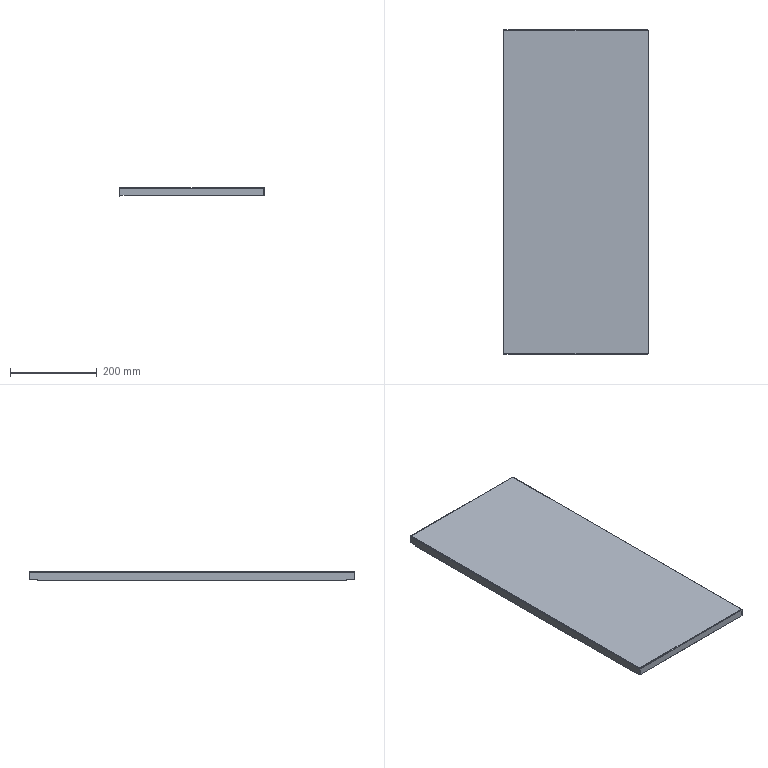Part | SolidWorks | features BaseBody 1 | 1 solid | 44 faces | box 336 x 750 x 20 mm | volume 346440 mm3 | plane 32 | cylinder 8 | spline 4 | commonest cylinder face diameters 1 x4 3.4 x4
STEP:
#1=CARTESIAN_POINT('',(-168.,-375.,-18.));
#2=VERTEX_POINT('',#1);
#3=CARTESIAN_POINT('',(-168.,-357.,-18.));
#4=VERTEX_POINT('',#3);
#5=CARTESIAN_POINT('',(-168.,-375.,-18.));
#6=DIRECTION('',(0.,1.,0.));
#7=VECTOR('',#6,1000.);
#8=LINE('',#5,#7);
#9=EDGE_CURVE('',#2,#4,#8,.T.);
#10=ORIENTED_EDGE('',*,*,#9,.T.);
#11=CARTESIAN_POINT('',(-166.8,-357.,-18.));
#12=VERTEX_POINT('',#11);
#13=CARTESIAN_POINT('',(-166.8,-357.,-18.));
#14=DIRECTION('',(-1.,0.,0.));
#15=VECTOR('',#14,1000.);
#16=LINE('',#13,#15);
#17=EDGE_CURVE('',#12,#4,#16,.T.);
#18=ORIENTED_EDGE('',*,*,#17,.F.);
#19=CARTESIAN_POINT('',(-166.8,-375.,-18.));
#20=VERTEX_POINT('',#19);
#21=CARTESIAN_POINT('',(-166.8,-375.,-18.));
#22=DIRECTION('',(0.,1.,0.));
#23=VECTOR('',#22,1000.);
#24=LINE('',#21,#23);
#25=EDGE_CURVE('',#20,#12,#24,.T.);
#26=ORIENTED_EDGE('',*,*,#25,.F.);
#27=CARTESIAN_POINT('',(-166.8,-375.,-18.));
#28=DIRECTION('',(-1.,0.,0.));
#29=VECTOR('',#28,1000.);
#30=LINE('',#27,#29);
#31=EDGE_CURVE('',#20,#2,#30,.T.);
#32=ORIENTED_EDGE('',*,*,#31,.T.);
#33=EDGE_LOOP('',(#10,#18,#26,#32));
#34=FACE_OUTER_BOUND('',#33,.T.);
#35=CARTESIAN_POINT('',(-166.8,-375.,-18.));
#36=DIRECTION('',(0.,0.,1.));
#37=DIRECTION('',(1.,0.,0.));
#38=AXIS2_PLACEMENT_3D('',#35,#36,#37);
#39=PLANE('',#38);
#40=ADVANCED_FACE('',(#34),#39,.F.);
#41=CARTESIAN_POINT('',(-168.,-357.,-20.));
#42=VERTEX_POINT('',#41);
#43=CARTESIAN_POINT('',(-168.,-357.,-20.));
#44=DIRECTION('',(0.,0.,-1.));
#45=VECTOR('',#44,1000.);
#46=LINE('',#43,#45);
#47=EDGE_CURVE('',#4,#42,#46,.T.);
#48=ORIENTED_EDGE('',*,*,#47,.T.);
#49=CARTESIAN_POINT('',(-166.8,-357.,-20.));
#50=VERTEX_POINT('',#49);
#51=CARTESIAN_POINT('',(-166.8,-357.,-20.));
#52=DIRECTION('',(-1.,0.,0.));
#53=VECTOR('',#52,1000.);
#54=LINE('',#51,#53);
#55=EDGE_CURVE('',#50,#42,#54,.T.);
#56=ORIENTED_EDGE('',*,*,#55,.F.);
#57=CARTESIAN_POINT('',(-166.8,-357.,-20.));
#58=DIRECTION('',(0.,0.,-1.));
#59=VECTOR('',#58,1000.);
#60=LINE('',#57,#59);
#61=EDGE_CURVE('',#12,#50,#60,.T.);
#62=ORIENTED_EDGE('',*,*,#61,.F.);
#63=ORIENTED_EDGE('',*,*,#17,.T.);
#64=EDGE_LOOP('',(#48,#56,#62,#63));
#65=FACE_OUTER_BOUND('',#64,.T.);
#66=CARTESIAN_POINT('',(-166.8,-357.,-20.));
#67=DIRECTION('',(0.,1.,0.));
#68=DIRECTION('',(1.,0.,0.));
#69=AXIS2_PLACEMENT_3D('',#66,#67,#68);
#70=PLANE('',#69);
#71=ADVANCED_FACE('',(#65),#70,.F.);
#72=CARTESIAN_POINT('',(-168.,357.,-20.));
#73=VERTEX_POINT('',#72);
#74=CARTESIAN_POINT('',(-168.,357.,-18.));
#75=VERTEX_POINT('',#74);
#76=CARTESIAN_POINT('',(-168.,357.,-20.));
#77=DIRECTION('',(0.,0.,1.));
#78=VECTOR('',#77,1000.);
#79=LINE('',#76,#78);
#80=EDGE_CURVE('',#73,#75,#79,.T.);
#81=ORIENTED_EDGE('',*,*,#80,.T.);
#82=CARTESIAN_POINT('',(-166.8,357.,-18.));
#83=VERTEX_POINT('',#82);
#84=CARTESIAN_POINT('',(-166.8,357.,-18.));
#85=DIRECTION('',(-1.,0.,0.));
#86=VECTOR('',#85,1000.);
#87=LINE('',#84,#86);
#88=EDGE_CURVE('',#83,#75,#87,.T.);
#89=ORIENTED_EDGE('',*,*,#88,.F.);
#90=CARTESIAN_POINT('',(-166.8,357.,-20.));
#91=VERTEX_POINT('',#90);
#92=CARTESIAN_POINT('',(-166.8,357.,-20.));
#93=DIRECTION('',(0.,0.,1.));
#94=VECTOR('',#93,1000.);
#95=LINE('',#92,#94);
#96=EDGE_CURVE('',#91,#83,#95,.T.);
#97=ORIENTED_EDGE('',*,*,#96,.F.);
#98=CARTESIAN_POINT('',(-166.8,357.,-20.));
#99=DIRECTION('',(-1.,0.,0.));
#100=VECTOR('',#99,1000.);
#101=LINE('',#98,#100);
#102=EDGE_CURVE('',#91,#73,#101,.T.);
#103=ORIENTED_EDGE('',*,*,#102,.T.);
#104=EDGE_LOOP('',(#81,#89,#97,#103));
#105=FACE_OUTER_BOUND('',#104,.T.);
#106=CARTESIAN_POINT('',(-166.8,357.,-20.));
#107=DIRECTION('',(0.,-1.,0.));
#108=DIRECTION('',(0.,0.,-1.));
#109=AXIS2_PLACEMENT_3D('',#106,#107,#108);
#110=PLANE('',#109);
#111=ADVANCED_FACE('',(#105),#110,.F.);
#112=CARTESIAN_POINT('',(-168.,375.,-18.));
#113=VERTEX_POINT('',#112);
#114=CARTESIAN_POINT('',(-168.,375.,-18.));
#115=DIRECTION('',(0.,1.,0.));
#116=VECTOR('',#115,1000.);
#117=LINE('',#114,#116);
#118=EDGE_CURVE('',#75,#113,#117,.T.);
#119=ORIENTED_EDGE('',*,*,#118,.T.);
#120=CARTESIAN_POINT('',(-166.8,375.,-18.));
#121=VERTEX_POINT('',#120);
#122=CARTESIAN_POINT('',(-166.8,375.,-18.));
#123=DIRECTION('',(-1.,0.,0.));
#124=VECTOR('',#123,1000.);
#125=LINE('',#122,#124);
#126=EDGE_CURVE('',#121,#113,#125,.T.);
#127=ORIENTED_EDGE('',*,*,#126,.F.);
#128=CARTESIAN_POINT('',(-166.8,375.,-18.));
#129=DIRECTION('',(0.,1.,0.));
#130=VECTOR('',#129,1000.);
#131=LINE('',#128,#130);
#132=EDGE_CURVE('',#83,#121,#131,.T.);
#133=ORIENTED_EDGE('',*,*,#132,.F.);
#134=ORIENTED_EDGE('',*,*,#88,.T.);
#135=EDGE_LOOP('',(#119,#127,#133,#134));
#136=FACE_OUTER_BOUND('',#135,.T.);
#137=CARTESIAN_POINT('',(-166.8,375.,-18.));
#138=DIRECTION('',(0.,0.,1.));
#139=DIRECTION('',(1.,0.,0.));
#140=AXIS2_PLACEMENT_3D('',#137,#138,#139);
#141=PLANE('',#140);
#142=ADVANCED_FACE('',(#136),#141,.F.);
#143=CARTESIAN_POINT('',(166.093,375.,-18.));
#144=VERTEX_POINT('',#143);
#145=CARTESIAN_POINT('',(166.093,373.8,-18.));
#146=VERTEX_POINT('',#145);
#147=CARTESIAN_POINT('',(166.093,375.,-18.));
#148=DIRECTION('',(0.,-1.,0.));
#149=VECTOR('',#148,1000.);
#150=LINE('',#147,#149);
#151=EDGE_CURVE('',#144,#146,#150,.T.);
#152=ORIENTED_EDGE('',*,*,#151,.F.);
#153=CARTESIAN_POINT('',(166.093,375.,-1.7));
#154=VERTEX_POINT('',#153);
#155=CARTESIAN_POINT('',(166.093,375.,0.));
#156=DIRECTION('',(0.,0.,-1.));
#157=VECTOR('',#156,1000.);
#158=LINE('',#155,#157);
#159=EDGE_CURVE('',#154,#144,#158,.T.);
#160=ORIENTED_EDGE('',*,*,#159,.F.);
#161=CARTESIAN_POINT('',(166.093,373.8,-1.7));
#162=VERTEX_POINT('',#161);
#163=CARTESIAN_POINT('',(166.093,373.8,-1.7));
#164=DIRECTION('',(0.,-1.,0.));
#165=VECTOR('',#164,1000.);
#166=LINE('',#163,#165);
#167=EDGE_CURVE('',#154,#162,#166,.T.);
#168=ORIENTED_EDGE('',*,*,#167,.T.);
#169=CARTESIAN_POINT('',(166.093,373.8,-1.2));
#170=DIRECTION('',(0.,0.,-1.));
#171=VECTOR('',#170,1000.);
#172=LINE('',#169,#171);
#173=EDGE_CURVE('',#162,#146,#172,.T.);
#174=ORIENTED_EDGE('',*,*,#173,.T.);
#175=EDGE_LOOP('',(#152,#160,#168,#174));
#176=FACE_OUTER_BOUND('',#175,.T.);
#177=CARTESIAN_POINT('',(166.093,373.8,-1.2));
#178=DIRECTION('',(-1.,0.,0.));
#179=DIRECTION('',(0.,0.,1.));
#180=AXIS2_PLACEMENT_3D('',#177,#178,#179);
#181=PLANE('',#180);
#182=ADVANCED_FACE('',(#176),#181,.F.);
#183=CARTESIAN_POINT('',(-166.3,375.,-18.));
#184=VERTEX_POINT('',#183);
#185=CARTESIAN_POINT('',(0.,375.,-18.));
#186=DIRECTION('',(-1.,0.,0.));
#187=VECTOR('',#186,1000.);
#188=LINE('',#185,#187);
#189=EDGE_CURVE('',#144,#184,#188,.T.);
#190=ORIENTED_EDGE('',*,*,#189,.F.);
#191=ORIENTED_EDGE('',*,*,#151,.T.);
#192=CARTESIAN_POINT('',(-166.3,373.8,-18.));
#193=VERTEX_POINT('',#192);
#194=CARTESIAN_POINT('',(-166.3,373.8,-18.));
#195=DIRECTION('',(-1.,0.,0.));
#196=VECTOR('',#195,1000.);
#197=LINE('',#194,#196);
#198=EDGE_CURVE('',#146,#193,#197,.T.);
#199=ORIENTED_EDGE('',*,*,#198,.T.);
#200=CARTESIAN_POINT('',(-166.3,375.,-18.));
#201=DIRECTION('',(0.,-1.,0.));
#202=VECTOR('',#201,1000.);
#203=LINE('',#200,#202);
#204=EDGE_CURVE('',#184,#193,#203,.T.);
#205=ORIENTED_EDGE('',*,*,#204,.F.);
#206=EDGE_LOOP('',(#190,#191,#199,#205));
#207=FACE_OUTER_BOUND('',#206,.T.);
#208=CARTESIAN_POINT('',(-166.3,375.,-18.));
#209=DIRECTION('',(0.,0.,1.));
#210=DIRECTION('',(0.,-1.,0.));
#211=AXIS2_PLACEMENT_3D('',#208,#209,#210);
#212=PLANE('',#211);
#213=ADVANCED_FACE('',(#207),#212,.F.);
#214=ORIENTED_EDGE('',*,*,#173,.F.);
#215=CARTESIAN_POINT('',(-166.3,373.8,-1.7));
#216=VERTEX_POINT('',#215);
#217=CARTESIAN_POINT('',(-166.3,373.8,-1.7));
#218=DIRECTION('',(1.,0.,0.));
#219=VECTOR('',#218,1000.);
#220=LINE('',#217,#219);
#221=EDGE_CURVE('',#216,#162,#220,.T.);
#222=ORIENTED_EDGE('',*,*,#221,.F.);
#223=CARTESIAN_POINT('',(-166.3,373.8,-1.2));
#224=DIRECTION('',(0.,0.,1.));
#225=VECTOR('',#224,1000.);
#226=LINE('',#223,#225);
#227=EDGE_CURVE('',#193,#216,#226,.T.);
#228=ORIENTED_EDGE('',*,*,#227,.F.);
#229=ORIENTED_EDGE('',*,*,#198,.F.);
#230=EDGE_LOOP('',(#214,#222,#228,#229));
#231=FACE_OUTER_BOUND('',#230,.T.);
#232=CARTESIAN_POINT('',(0.,373.8,0.));
#233=DIRECTION('',(0.,-1.,0.));
#234=DIRECTION('',(0.,0.,-1.));
#235=AXIS2_PLACEMENT_3D('',#232,#233,#234);
#236=PLANE('',#235);
#237=ADVANCED_FACE('',(#231),#236,.T.);
#238=CARTESIAN_POINT('',(-166.3,375.,-1.7));
#239=VERTEX_POINT('',#238);
#240=CARTESIAN_POINT('',(-166.3,375.,-1.7));
#241=DIRECTION('',(-1.,0.,0.));
#242=VECTOR('',#241,1000.);
#243=LINE('',#240,#242);
#244=EDGE_CURVE('',#154,#239,#243,.T.);
#245=ORIENTED_EDGE('',*,*,#244,.F.);
#246=ORIENTED_EDGE('',*,*,#159,.T.);
#247=ORIENTED_EDGE('',*,*,#189,.T.);
#248=CARTESIAN_POINT('',(-166.3,375.,0.));
#249=DIRECTION('',(0.,0.,1.));
#250=VECTOR('',#249,1000.);
#251=LINE('',#248,#250);
#252=EDGE_CURVE('',#184,#239,#251,.T.);
#253=ORIENTED_EDGE('',*,*,#252,.T.);
#254=EDGE_LOOP('',(#245,#246,#247,#253));
#255=FACE_OUTER_BOUND('',#254,.T.);
#256=CARTESIAN_POINT('',(0.,375.,0.));
#257=DIRECTION('',(0.,-1.,0.));
#258=DIRECTION('',(0.,0.,-1.));
#259=AXIS2_PLACEMENT_3D('',#256,#257,#258);
#260=PLANE('',#259);
#261=ADVANCED_FACE('',(#255),#260,.F.);
#262=CARTESIAN_POINT('',(-166.3,375.,-1.7));
#263=DIRECTION('',(0.,1.,0.));
#264=VECTOR('',#263,1000.);
#265=LINE('',#262,#264);
#266=EDGE_CURVE('',#216,#239,#265,.T.);
#267=ORIENTED_EDGE('',*,*,#266,.T.);
#268=ORIENTED_EDGE('',*,*,#252,.F.);
#269=ORIENTED_EDGE('',*,*,#204,.T.);
#270=ORIENTED_EDGE('',*,*,#227,.T.);
#271=EDGE_LOOP('',(#267,#268,#269,#270));
#272=FACE_OUTER_BOUND('',#271,.T.);
#273=CARTESIAN_POINT('',(-166.3,375.,-1.2));
#274=DIRECTION('',(1.,0.,0.));
#275=DIRECTION('',(0.,1.,0.));
#276=AXIS2_PLACEMENT_3D('',#273,#274,#275);
#277=PLANE('',#276);
#278=ADVANCED_FACE('',(#272),#277,.F.);
#279=CARTESIAN_POINT('',(166.3,373.3,-1.2));
#280=VERTEX_POINT('',#279);
#281=CARTESIAN_POINT('',(-166.3,373.3,-1.2));
#282=VERTEX_POINT('',#281);
#283=CARTESIAN_POINT('',(166.3,373.3,-1.2));
#284=DIRECTION('',(-1.,0.,0.));
#285=VECTOR('',#284,1000.);
#286=LINE('',#283,#285);
#287=EDGE_CURVE('',#280,#282,#286,.T.);
#288=ORIENTED_EDGE('',*,*,#287,.T.);
#289=CARTESIAN_POINT('',(-166.3,373.3,-1.7));
#290=DIRECTION('',(-1.,0.,0.));
#291=DIRECTION('',(0.,0.,-1.));
#292=AXIS2_PLACEMENT_3D('',#289,#290,#291);
#293=CIRCLE('',#292,0.5);
#294=EDGE_CURVE('',#282,#216,#293,.T.);
#295=ORIENTED_EDGE('',*,*,#294,.T.);
#296=ORIENTED_EDGE('',*,*,#221,.T.);
#297=CARTESIAN_POINT('',(166.093,373.8,-1.7));
#298=CARTESIAN_POINT('',(166.127,373.8,-1.569));
#299=CARTESIAN_POINT('',(166.162,373.746,-1.439));
#300=CARTESIAN_POINT('',(166.231,373.561,-1.254));
#301=CARTESIAN_POINT('',(166.265,373.431,-1.2));
#302=CARTESIAN_POINT('',(166.3,373.3,-1.2));
#303=B_SPLINE_CURVE_WITH_KNOTS('',3,(#297,#298,#299,#300,#301,#302),.UNSPECIFIED.,.F.,.F.,(4,2,4),(0.,0.5,1.),.UNSPECIFIED.);
#304=EDGE_CURVE('',#162,#280,#303,.T.);
#305=ORIENTED_EDGE('',*,*,#304,.T.);
#306=EDGE_LOOP('',(#288,#295,#296,#305));
#307=FACE_OUTER_BOUND('',#306,.T.);
#308=CARTESIAN_POINT('',(166.3,373.3,-1.7));
#309=DIRECTION('',(1.,0.,0.));
#310=DIRECTION('',(0.,1.,0.));
#311=AXIS2_PLACEMENT_3D('',#308,#309,#310);
#312=CYLINDRICAL_SURFACE('',#311,0.5);
#313=ADVANCED_FACE('',(#307),#312,.F.);
#314=CARTESIAN_POINT('',(166.3,373.3,0.));
#315=VERTEX_POINT('',#314);
#316=CARTESIAN_POINT('',(-166.3,373.3,0.));
#317=VERTEX_POINT('',#316);
#318=CARTESIAN_POINT('',(166.3,373.3,0.));
#319=DIRECTION('',(-1.,0.,0.));
#320=VECTOR('',#319,1000.);
#321=LINE('',#318,#320);
#322=EDGE_CURVE('',#315,#317,#321,.T.);
#323=ORIENTED_EDGE('',*,*,#322,.F.);
#324=CARTESIAN_POINT('',(166.093,375.,-1.7));
#325=CARTESIAN_POINT('',(166.11,375.,-1.477));
#326=CARTESIAN_POINT('',(166.127,374.956,-1.255));
#327=CARTESIAN_POINT('',(166.162,374.785,-0.8438));
#328=CARTESIAN_POINT('',(166.179,374.659,-0.6553));
#329=CARTESIAN_POINT('',(166.214,374.345,-0.3406));
#330=CARTESIAN_POINT('',(166.231,374.156,-0.2146));
#331=CARTESIAN_POINT('',(166.265,373.745,-0.04425));
#332=CARTESIAN_POINT('',(166.283,373.523,0.));
#333=CARTESIAN_POINT('',(166.3,373.3,0.));
#334=B_SPLINE_CURVE_WITH_KNOTS('',3,(#324,#325,#326,#327,#328,#329,#330,#331,#332,#333),.UNSPECIFIED.,.F.,.F.,(4,2,2,2,4),(0.,0.25,0.5,0.75,1.),.UNSPECIFIED.);
#335=EDGE_CURVE('',#154,#315,#334,.T.);
#336=ORIENTED_EDGE('',*,*,#335,.F.);
#337=ORIENTED_EDGE('',*,*,#244,.T.);
#338=CARTESIAN_POINT('',(-166.3,373.3,-1.7));
#339=DIRECTION('',(-1.,0.,0.));
#340=DIRECTION('',(0.,0.,-1.));
#341=AXIS2_PLACEMENT_3D('',#338,#339,#340);
#342=CIRCLE('',#341,1.7);
#343=EDGE_CURVE('',#317,#239,#342,.T.);
#344=ORIENTED_EDGE('',*,*,#343,.F.);
#345=EDGE_LOOP('',(#323,#336,#337,#344));
#346=FACE_OUTER_BOUND('',#345,.T.);
#347=CARTESIAN_POINT('',(166.3,373.3,-1.7));
#348=DIRECTION('',(1.,0.,0.));
#349=DIRECTION('',(0.,1.,0.));
#350=AXIS2_PLACEMENT_3D('',#347,#348,#349);
#351=CYLINDRICAL_SURFACE('',#350,1.7);
#352=ADVANCED_FACE('',(#346),#351,.T.);
#353=ORIENTED_EDGE('',*,*,#304,.F.);
#354=ORIENTED_EDGE('',*,*,#167,.F.);
#355=ORIENTED_EDGE('',*,*,#335,.T.);
#356=CARTESIAN_POINT('',(166.3,373.3,-1.2));
#357=DIRECTION('',(0.,0.,1.));
#358=VECTOR('',#357,1000.);
#359=LINE('',#356,#358);
#360=EDGE_CURVE('',#280,#315,#359,.T.);
#361=ORIENTED_EDGE('',*,*,#360,.F.);
#362=EDGE_LOOP('',(#353,#354,#355,#361));
#363=FACE_OUTER_BOUND('',#362,.T.);
#364=CARTESIAN_POINT('',(166.093,375.012,-1.7));
#365=CARTESIAN_POINT('',(166.11,375.012,-1.476));
#366=CARTESIAN_POINT('',(166.127,374.967,-1.252));
#367=CARTESIAN_POINT('',(166.162,374.796,-0.8378));
#368=CARTESIAN_POINT('',(166.179,374.669,-0.6479));
#369=CARTESIAN_POINT('',(166.214,374.352,-0.331));
#370=CARTESIAN_POINT('',(166.231,374.162,-0.2041));
#371=CARTESIAN_POINT('',(166.265,373.748,-0.03256));
#372=CARTESIAN_POINT('',(166.283,373.524,0.012));
#373=CARTESIAN_POINT('',(166.3,373.3,0.012));
#374=CARTESIAN_POINT('',(166.093,375.,-1.7));
#375=CARTESIAN_POINT('',(166.11,375.,-1.477));
#376=CARTESIAN_POINT('',(166.127,374.956,-1.255));
#377=CARTESIAN_POINT('',(166.162,374.785,-0.8438));
#378=CARTESIAN_POINT('',(166.179,374.659,-0.6553));
#379=CARTESIAN_POINT('',(166.214,374.345,-0.3406));
#380=CARTESIAN_POINT('',(166.231,374.156,-0.2146));
#381=CARTESIAN_POINT('',(166.265,373.745,-0.04425));
#382=CARTESIAN_POINT('',(166.283,373.523,0.));
#383=CARTESIAN_POINT('',(166.3,373.3,0.));
#384=CARTESIAN_POINT('',(166.093,373.8,-1.7));
#385=CARTESIAN_POINT('',(166.11,373.8,-1.635));
#386=CARTESIAN_POINT('',(166.127,373.787,-1.569));
#387=CARTESIAN_POINT('',(166.162,373.737,-1.448));
#388=CARTESIAN_POINT('',(166.179,373.7,-1.393));
#389=CARTESIAN_POINT('',(166.214,373.607,-1.3));
#390=CARTESIAN_POINT('',(166.231,373.552,-1.263));
#391=CARTESIAN_POINT('',(166.265,373.431,-1.213));
#392=CARTESIAN_POINT('',(166.283,373.365,-1.2));
#393=CARTESIAN_POINT('',(166.3,373.3,-1.2));
#394=CARTESIAN_POINT('',(166.093,373.788,-1.7));
#395=CARTESIAN_POINT('',(166.11,373.788,-1.636));
#396=CARTESIAN_POINT('',(166.127,373.775,-1.572));
#397=CARTESIAN_POINT('',(166.162,373.726,-1.454));
#398=CARTESIAN_POINT('',(166.179,373.69,-1.4));
#399=CARTESIAN_POINT('',(166.214,373.6,-1.31));
#400=CARTESIAN_POINT('',(166.231,373.546,-1.274));
#401=CARTESIAN_POINT('',(166.265,373.428,-1.225));
#402=CARTESIAN_POINT('',(166.283,373.364,-1.212));
#403=CARTESIAN_POINT('',(166.3,373.3,-1.212));
#404=B_SPLINE_SURFACE_WITH_KNOTS('',1,3,((#364,#365,#366,#367,#368,#369,#370,#371,#372,#373),(#374,#375,#376,#377,#378,#379,#380,#381,#382,#383),(#384,#385,#386,#387,#388,#389,#390,#391,#392,#393),(#394,#395,#396,#397,#398,#399,#400,#401,#402,#403)),.UNSPECIFIED.,.F.,.F.,.F.,(2,1,1,2),(4,2,2,2,4),(-0.01,0.,1.,1.01),(0.,0.25,0.5,0.75,1.),.UNSPECIFIED.);
#405=ADVANCED_FACE('',(#363),#404,.F.);
#406=ORIENTED_EDGE('',*,*,#266,.F.);
#407=ORIENTED_EDGE('',*,*,#294,.F.);
#408=CARTESIAN_POINT('',(-166.3,373.3,-1.2));
#409=DIRECTION('',(0.,0.,1.));
#410=VECTOR('',#409,1000.);
#411=LINE('',#408,#410);
#412=EDGE_CURVE('',#282,#317,#411,.T.);
#413=ORIENTED_EDGE('',*,*,#412,.T.);
#414=ORIENTED_EDGE('',*,*,#343,.T.);
#415=EDGE_LOOP('',(#406,#407,#413,#414));
#416=FACE_OUTER_BOUND('',#415,.T.);
#417=CARTESIAN_POINT('',(-166.3,373.3,-1.7));
#418=DIRECTION('',(-1.,0.,0.));
#419=DIRECTION('',(0.,0.,1.));
#420=AXIS2_PLACEMENT_3D('',#417,#418,#419);
#421=PLANE('',#420);
#422=ADVANCED_FACE('',(#416),#421,.T.);
#423=CARTESIAN_POINT('',(168.,-373.093,-18.));
#424=VERTEX_POINT('',#423);
#425=CARTESIAN_POINT('',(166.8,-373.093,-18.));
#426=VERTEX_POINT('',#425);
#427=CARTESIAN_POINT('',(168.,-373.093,-18.));
#428=DIRECTION('',(-1.,0.,0.));
#429=VECTOR('',#428,1000.);
#430=LINE('',#427,#429);
#431=EDGE_CURVE('',#424,#426,#430,.T.);
#432=ORIENTED_EDGE('',*,*,#431,.F.);
#433=CARTESIAN_POINT('',(168.,-373.093,-1.7));
#434=VERTEX_POINT('',#433);
#435=CARTESIAN_POINT('',(168.,-373.093,0.));
#436=DIRECTION('',(0.,0.,-1.));
#437=VECTOR('',#436,1000.);
#438=LINE('',#435,#437);
#439=EDGE_CURVE('',#434,#424,#438,.T.);
#440=ORIENTED_EDGE('',*,*,#439,.F.);
#441=CARTESIAN_POINT('',(166.8,-373.093,-1.7));
#442=VERTEX_POINT('',#441);
#443=CARTESIAN_POINT('',(166.8,-373.093,-1.7));
#444=DIRECTION('',(-1.,0.,0.));
#445=VECTOR('',#444,1000.);
#446=LINE('',#443,#445);
#447=EDGE_CURVE('',#434,#442,#446,.T.);
#448=ORIENTED_EDGE('',*,*,#447,.T.);
#449=CARTESIAN_POINT('',(166.8,-373.093,-1.2));
#450=DIRECTION('',(0.,0.,-1.));
#451=VECTOR('',#450,1000.);
#452=LINE('',#449,#451);
#453=EDGE_CURVE('',#442,#426,#452,.T.);
#454=ORIENTED_EDGE('',*,*,#453,.T.);
#455=EDGE_LOOP('',(#432,#440,#448,#454));
#456=FACE_OUTER_BOUND('',#455,.T.);
#457=CARTESIAN_POINT('',(166.8,-373.093,-1.2));
#458=DIRECTION('',(0.,1.,0.));
#459=DIRECTION('',(0.,0.,-1.));
#460=AXIS2_PLACEMENT_3D('',#457,#458,#459);
#461=PLANE('',#460);
#462=ADVANCED_FACE('',(#456),#461,.F.);
#463=CARTESIAN_POINT('',(168.,373.093,-18.));
#464=VERTEX_POINT('',#463);
#465=CARTESIAN_POINT('',(166.8,373.093,-18.));
#466=VERTEX_POINT('',#465);
#467=CARTESIAN_POINT('',(166.8,373.093,-18.));
#468=DIRECTION('',(-1.,0.,0.));
#469=VECTOR('',#468,1000.);
#470=LINE('',#467,#469);
#471=EDGE_CURVE('',#464,#466,#470,.T.);
#472=ORIENTED_EDGE('',*,*,#471,.F.);
#473=CARTESIAN_POINT('',(168.,0.,-18.));
#474=DIRECTION('',(0.,1.,0.));
#475=VECTOR('',#474,1000.);
#476=LINE('',#473,#475);
#477=EDGE_CURVE('',#424,#464,#476,.T.);
#478=ORIENTED_EDGE('',*,*,#477,.F.);
#479=ORIENTED_EDGE('',*,*,#431,.T.);
#480=CARTESIAN_POINT('',(166.8,375.,-18.));
#481=DIRECTION('',(0.,1.,0.));
#482=VECTOR('',#481,1000.);
#483=LINE('',#480,#482);
#484=EDGE_CURVE('',#426,#466,#483,.T.);
#485=ORIENTED_EDGE('',*,*,#484,.T.);
#486=EDGE_LOOP('',(#472,#478,#479,#485));
#487=FACE_OUTER_BOUND('',#486,.T.);
#488=CARTESIAN_POINT('',(168.,375.,-18.));
#489=DIRECTION('',(0.,0.,1.));
#490=DIRECTION('',(1.,0.,0.));
#491=AXIS2_PLACEMENT_3D('',#488,#489,#490);
#492=PLANE('',#491);
#493=ADVANCED_FACE('',(#487),#492,.F.);
#494=CARTESIAN_POINT('',(166.8,373.093,-1.7));
#495=VERTEX_POINT('',#494);
#496=CARTESIAN_POINT('',(166.8,375.,-1.7));
#497=DIRECTION('',(0.,-1.,0.));
#498=VECTOR('',#497,1000.);
#499=LINE('',#496,#498);
#500=EDGE_CURVE('',#495,#442,#499,.T.);
#501=ORIENTED_EDGE('',*,*,#500,.F.);
#502=CARTESIAN_POINT('',(166.8,373.093,0.));
#503=DIRECTION('',(0.,0.,-1.));
#504=VECTOR('',#503,1000.);
#505=LINE('',#502,#504);
#506=EDGE_CURVE('',#495,#466,#505,.T.);
#507=ORIENTED_EDGE('',*,*,#506,.T.);
#508=ORIENTED_EDGE('',*,*,#484,.F.);
#509=ORIENTED_EDGE('',*,*,#453,.F.);
#510=EDGE_LOOP('',(#501,#507,#508,#509));
#511=FACE_OUTER_BOUND('',#510,.T.);
#512=CARTESIAN_POINT('',(166.8,0.,0.));
#513=DIRECTION('',(-1.,0.,0.));
#514=DIRECTION('',(0.,0.,1.));
#515=AXIS2_PLACEMENT_3D('',#512,#513,#514);
#516=PLANE('',#515);
#517=ADVANCED_FACE('',(#511),#516,.T.);
#518=CARTESIAN_POINT('',(168.,373.093,-1.7));
#519=VERTEX_POINT('',#518);
#520=CARTESIAN_POINT('',(168.,373.093,-1.2));
#521=DIRECTION('',(0.,0.,-1.));
#522=VECTOR('',#521,1000.);
#523=LINE('',#520,#522);
#524=EDGE_CURVE('',#519,#464,#523,.T.);
#525=ORIENTED_EDGE('',*,*,#524,.F.);
#526=CARTESIAN_POINT('',(168.,375.,-1.7));
#527=DIRECTION('',(0.,1.,0.));
#528=VECTOR('',#527,1000.);
#529=LINE('',#526,#528);
#530=EDGE_CURVE('',#434,#519,#529,.T.);
#531=ORIENTED_EDGE('',*,*,#530,.F.);
#532=ORIENTED_EDGE('',*,*,#439,.T.);
#533=ORIENTED_EDGE('',*,*,#477,.T.);
#534=EDGE_LOOP('',(#525,#531,#532,#533));
#535=FACE_OUTER_BOUND('',#534,.T.);
#536=CARTESIAN_POINT('',(168.,0.,0.));
#537=DIRECTION('',(-1.,0.,0.));
#538=DIRECTION('',(0.,0.,1.));
#539=AXIS2_PLACEMENT_3D('',#536,#537,#538);
#540=PLANE('',#539);
#541=ADVANCED_FACE('',(#535),#540,.F.);
#542=ORIENTED_EDGE('',*,*,#524,.T.);
#543=ORIENTED_EDGE('',*,*,#471,.T.);
#544=ORIENTED_EDGE('',*,*,#506,.F.);
#545=CARTESIAN_POINT('',(166.8,373.093,-1.7));
#546=DIRECTION('',(-1.,0.,0.));
#547=VECTOR('',#546,1000.);
#548=LINE('',#545,#547);
#549=EDGE_CURVE('',#519,#495,#548,.T.);
#550=ORIENTED_EDGE('',*,*,#549,.F.);
#551=EDGE_LOOP('',(#542,#543,#544,#550));
#552=FACE_OUTER_BOUND('',#551,.T.);
#553=CARTESIAN_POINT('',(166.8,373.093,-1.2));
#554=DIRECTION('',(0.,1.,0.));
#555=DIRECTION('',(0.,0.,-1.));
#556=AXIS2_PLACEMENT_3D('',#553,#554,#555);
#557=PLANE('',#556);
#558=ADVANCED_FACE('',(#552),#557,.T.);
#559=CARTESIAN_POINT('',(166.3,-373.3,-1.2));
#560=VERTEX_POINT('',#559);
#561=CARTESIAN_POINT('',(166.3,-373.3,-1.2));
#562=DIRECTION('',(0.,1.,0.));
#563=VECTOR('',#562,1000.);
#564=LINE('',#561,#563);
#565=EDGE_CURVE('',#560,#280,#564,.T.);
#566=ORIENTED_EDGE('',*,*,#565,.T.);
#567=CARTESIAN_POINT('',(166.3,373.3,-1.2));
#568=CARTESIAN_POINT('',(166.431,373.265,-1.2));
#569=CARTESIAN_POINT('',(166.561,373.231,-1.254));
#570=CARTESIAN_POINT('',(166.746,373.162,-1.439));
#571=CARTESIAN_POINT('',(166.8,373.127,-1.569));
#572=CARTESIAN_POINT('',(166.8,373.093,-1.7));
#573=B_SPLINE_CURVE_WITH_KNOTS('',3,(#567,#568,#569,#570,#571,#572),.UNSPECIFIED.,.F.,.F.,(4,2,4),(0.,0.5,1.),.UNSPECIFIED.);
#574=EDGE_CURVE('',#280,#495,#573,.T.);
#575=ORIENTED_EDGE('',*,*,#574,.T.);
#576=ORIENTED_EDGE('',*,*,#500,.T.);
#577=CARTESIAN_POINT('',(166.8,-373.093,-1.7));
#578=CARTESIAN_POINT('',(166.8,-373.127,-1.569));
#579=CARTESIAN_POINT('',(166.746,-373.162,-1.439));
#580=CARTESIAN_POINT('',(166.561,-373.231,-1.254));
#581=CARTESIAN_POINT('',(166.431,-373.265,-1.2));
#582=CARTESIAN_POINT('',(166.3,-373.3,-1.2));
#583=B_SPLINE_CURVE_WITH_KNOTS('',3,(#577,#578,#579,#580,#581,#582),.UNSPECIFIED.,.F.,.F.,(4,2,4),(0.,0.5,1.),.UNSPECIFIED.);
#584=EDGE_CURVE('',#442,#560,#583,.T.);
#585=ORIENTED_EDGE('',*,*,#584,.T.);
#586=EDGE_LOOP('',(#566,#575,#576,#585));
#587=FACE_OUTER_BOUND('',#586,.T.);
#588=CARTESIAN_POINT('',(166.3,-373.3,-1.7));
#589=DIRECTION('',(0.,-1.,0.));
#590=DIRECTION('',(1.,0.,0.));
#591=AXIS2_PLACEMENT_3D('',#588,#589,#590);
#592=CYLINDRICAL_SURFACE('',#591,0.5);
#593=ADVANCED_FACE('',(#587),#592,.F.);
#594=CARTESIAN_POINT('',(166.3,-373.3,0.));
#595=VERTEX_POINT('',#594);
#596=CARTESIAN_POINT('',(166.3,-373.3,0.));
#597=DIRECTION('',(0.,1.,0.));
#598=VECTOR('',#597,1000.);
#599=LINE('',#596,#598);
#600=EDGE_CURVE('',#595,#315,#599,.T.);
#601=ORIENTED_EDGE('',*,*,#600,.F.);
#602=CARTESIAN_POINT('',(168.,-373.093,-1.7));
#603=CARTESIAN_POINT('',(168.,-373.11,-1.477));
#604=CARTESIAN_POINT('',(167.956,-373.127,-1.255));
#605=CARTESIAN_POINT('',(167.785,-373.162,-0.8438));
#606=CARTESIAN_POINT('',(167.659,-373.179,-0.6553));
#607=CARTESIAN_POINT('',(167.345,-373.214,-0.3406));
#608=CARTESIAN_POINT('',(167.156,-373.231,-0.2146));
#609=CARTESIAN_POINT('',(166.745,-373.265,-0.04425));
#610=CARTESIAN_POINT('',(166.523,-373.283,0.));
#611=CARTESIAN_POINT('',(166.3,-373.3,0.));
#612=B_SPLINE_CURVE_WITH_KNOTS('',3,(#602,#603,#604,#605,#606,#607,#608,#609,#610,#611),.UNSPECIFIED.,.F.,.F.,(4,2,2,2,4),(0.,0.25,0.5,0.75,1.),.UNSPECIFIED.);
#613=EDGE_CURVE('',#434,#595,#612,.T.);
#614=ORIENTED_EDGE('',*,*,#613,.F.);
#615=ORIENTED_EDGE('',*,*,#530,.T.);
#616=CARTESIAN_POINT('',(166.3,373.3,0.));
#617=CARTESIAN_POINT('',(166.523,373.283,0.));
#618=CARTESIAN_POINT('',(166.745,373.265,-0.04425));
#619=CARTESIAN_POINT('',(167.156,373.231,-0.2146));
#620=CARTESIAN_POINT('',(167.345,373.214,-0.3406));
#621=CARTESIAN_POINT('',(167.659,373.179,-0.6553));
#622=CARTESIAN_POINT('',(167.785,373.162,-0.8438));
#623=CARTESIAN_POINT('',(167.956,373.127,-1.255));
#624=CARTESIAN_POINT('',(168.,373.11,-1.477));
#625=CARTESIAN_POINT('',(168.,373.093,-1.7));
#626=B_SPLINE_CURVE_WITH_KNOTS('',3,(#616,#617,#618,#619,#620,#621,#622,#623,#624,#625),.UNSPECIFIED.,.F.,.F.,(4,2,2,2,4),(0.,0.25,0.5,0.75,1.),.UNSPECIFIED.);
#627=EDGE_CURVE('',#315,#519,#626,.T.);
#628=ORIENTED_EDGE('',*,*,#627,.F.);
#629=EDGE_LOOP('',(#601,#614,#615,#628));
#630=FACE_OUTER_BOUND('',#629,.T.);
#631=CARTESIAN_POINT('',(166.3,-373.3,-1.7));
#632=DIRECTION('',(0.,-1.,0.));
#633=DIRECTION('',(1.,0.,0.));
#634=AXIS2_PLACEMENT_3D('',#631,#632,#633);
#635=CYLINDRICAL_SURFACE('',#634,1.7);
#636=ADVANCED_FACE('',(#630),#635,.T.);
#637=ORIENTED_EDGE('',*,*,#584,.F.);
#638=ORIENTED_EDGE('',*,*,#447,.F.);
#639=ORIENTED_EDGE('',*,*,#613,.T.);
#640=CARTESIAN_POINT('',(166.3,-373.3,-1.2));
#641=DIRECTION('',(0.,0.,1.));
#642=VECTOR('',#641,1000.);
#643=LINE('',#640,#642);
#644=EDGE_CURVE('',#560,#595,#643,.T.);
#645=ORIENTED_EDGE('',*,*,#644,.F.);
#646=EDGE_LOOP('',(#637,#638,#639,#645));
#647=FACE_OUTER_BOUND('',#646,.T.);
#648=CARTESIAN_POINT('',(168.012,-373.093,-1.7));
#649=CARTESIAN_POINT('',(168.012,-373.11,-1.476));
#650=CARTESIAN_POINT('',(167.967,-373.127,-1.252));
#651=CARTESIAN_POINT('',(167.796,-373.162,-0.8378));
#652=CARTESIAN_POINT('',(167.669,-373.179,-0.6479));
#653=CARTESIAN_POINT('',(167.352,-373.214,-0.331));
#654=CARTESIAN_POINT('',(167.162,-373.231,-0.2041));
#655=CARTESIAN_POINT('',(166.748,-373.265,-0.03256));
#656=CARTESIAN_POINT('',(166.524,-373.283,0.012));
#657=CARTESIAN_POINT('',(166.3,-373.3,0.012));
#658=CARTESIAN_POINT('',(168.,-373.093,-1.7));
#659=CARTESIAN_POINT('',(168.,-373.11,-1.477));
#660=CARTESIAN_POINT('',(167.956,-373.127,-1.255));
#661=CARTESIAN_POINT('',(167.785,-373.162,-0.8438));
#662=CARTESIAN_POINT('',(167.659,-373.179,-0.6553));
#663=CARTESIAN_POINT('',(167.345,-373.214,-0.3406));
#664=CARTESIAN_POINT('',(167.156,-373.231,-0.2146));
#665=CARTESIAN_POINT('',(166.745,-373.265,-0.04425));
#666=CARTESIAN_POINT('',(166.523,-373.283,0.));
#667=CARTESIAN_POINT('',(166.3,-373.3,0.));
#668=CARTESIAN_POINT('',(166.8,-373.093,-1.7));
#669=CARTESIAN_POINT('',(166.8,-373.11,-1.635));
#670=CARTESIAN_POINT('',(166.787,-373.127,-1.569));
#671=CARTESIAN_POINT('',(166.737,-373.162,-1.448));
#672=CARTESIAN_POINT('',(166.7,-373.179,-1.393));
#673=CARTESIAN_POINT('',(166.607,-373.214,-1.3));
#674=CARTESIAN_POINT('',(166.552,-373.231,-1.263));
#675=CARTESIAN_POINT('',(166.431,-373.265,-1.213));
#676=CARTESIAN_POINT('',(166.365,-373.283,-1.2));
#677=CARTESIAN_POINT('',(166.3,-373.3,-1.2));
#678=CARTESIAN_POINT('',(166.788,-373.093,-1.7));
#679=CARTESIAN_POINT('',(166.788,-373.11,-1.636));
#680=CARTESIAN_POINT('',(166.775,-373.127,-1.572));
#681=CARTESIAN_POINT('',(166.726,-373.162,-1.454));
#682=CARTESIAN_POINT('',(166.69,-373.179,-1.4));
#683=CARTESIAN_POINT('',(166.6,-373.214,-1.31));
#684=CARTESIAN_POINT('',(166.546,-373.231,-1.274));
#685=CARTESIAN_POINT('',(166.428,-373.265,-1.225));
#686=CARTESIAN_POINT('',(166.364,-373.283,-1.212));
#687=CARTESIAN_POINT('',(166.3,-373.3,-1.212));
#688=B_SPLINE_SURFACE_WITH_KNOTS('',1,3,((#648,#649,#650,#651,#652,#653,#654,#655,#656,#657),(#658,#659,#660,#661,#662,#663,#664,#665,#666,#667),(#668,#669,#670,#671,#672,#673,#674,#675,#676,#677),(#678,#679,#680,#681,#682,#683,#684,#685,#686,#687)),.UNSPECIFIED.,.F.,.F.,.F.,(2,1,1,2),(4,2,2,2,4),(-0.01,0.,1.,1.01),(0.,0.25,0.5,0.75,1.),.UNSPECIFIED.);
#689=ADVANCED_FACE('',(#647),#688,.F.);
#690=ORIENTED_EDGE('',*,*,#549,.T.);
#691=ORIENTED_EDGE('',*,*,#574,.F.);
#692=ORIENTED_EDGE('',*,*,#360,.T.);
#693=ORIENTED_EDGE('',*,*,#627,.T.);
#694=EDGE_LOOP('',(#690,#691,#692,#693));
#695=FACE_OUTER_BOUND('',#694,.T.);
#696=CARTESIAN_POINT('',(166.3,373.3,0.012));
#697=CARTESIAN_POINT('',(166.524,373.283,0.012));
#698=CARTESIAN_POINT('',(166.748,373.265,-0.03256));
#699=CARTESIAN_POINT('',(167.162,373.231,-0.2041));
#700=CARTESIAN_POINT('',(167.352,373.214,-0.331));
#701=CARTESIAN_POINT('',(167.669,373.179,-0.6479));
#702=CARTESIAN_POINT('',(167.796,373.162,-0.8378));
#703=CARTESIAN_POINT('',(167.967,373.127,-1.252));
#704=CARTESIAN_POINT('',(168.012,373.11,-1.476));
#705=CARTESIAN_POINT('',(168.012,373.093,-1.7));
#706=CARTESIAN_POINT('',(166.3,373.3,0.));
#707=CARTESIAN_POINT('',(166.523,373.283,0.));
#708=CARTESIAN_POINT('',(166.745,373.265,-0.04425));
#709=CARTESIAN_POINT('',(167.156,373.231,-0.2146));
#710=CARTESIAN_POINT('',(167.345,373.214,-0.3406));
#711=CARTESIAN_POINT('',(167.659,373.179,-0.6553));
#712=CARTESIAN_POINT('',(167.785,373.162,-0.8438));
#713=CARTESIAN_POINT('',(167.956,373.127,-1.255));
#714=CARTESIAN_POINT('',(168.,373.11,-1.477));
#715=CARTESIAN_POINT('',(168.,373.093,-1.7));
#716=CARTESIAN_POINT('',(166.3,373.3,-1.2));
#717=CARTESIAN_POINT('',(166.365,373.283,-1.2));
#718=CARTESIAN_POINT('',(166.431,373.265,-1.213));
#719=CARTESIAN_POINT('',(166.552,373.231,-1.263));
#720=CARTESIAN_POINT('',(166.607,373.214,-1.3));
#721=CARTESIAN_POINT('',(166.7,373.179,-1.393));
#722=CARTESIAN_POINT('',(166.737,373.162,-1.448));
#723=CARTESIAN_POINT('',(166.787,373.127,-1.569));
#724=CARTESIAN_POINT('',(166.8,373.11,-1.635));
#725=CARTESIAN_POINT('',(166.8,373.093,-1.7));
#726=CARTESIAN_POINT('',(166.3,373.3,-1.212));
#727=CARTESIAN_POINT('',(166.364,373.283,-1.212));
#728=CARTESIAN_POINT('',(166.428,373.265,-1.225));
#729=CARTESIAN_POINT('',(166.546,373.231,-1.274));
#730=CARTESIAN_POINT('',(166.6,373.214,-1.31));
#731=CARTESIAN_POINT('',(166.69,373.179,-1.4));
#732=CARTESIAN_POINT('',(166.726,373.162,-1.454));
#733=CARTESIAN_POINT('',(166.775,373.127,-1.572));
#734=CARTESIAN_POINT('',(166.788,373.11,-1.636));
#735=CARTESIAN_POINT('',(166.788,373.093,-1.7));
#736=B_SPLINE_SURFACE_WITH_KNOTS('',1,3,((#696,#697,#698,#699,#700,#701,#702,#703,#704,#705),(#706,#707,#708,#709,#710,#711,#712,#713,#714,#715),(#716,#717,#718,#719,#720,#721,#722,#723,#724,#725),(#726,#727,#728,#729,#730,#731,#732,#733,#734,#735)),.UNSPECIFIED.,.F.,.F.,.F.,(2,1,1,2),(4,2,2,2,4),(-0.01,0.,1.,1.01),(0.,0.25,0.5,0.75,1.),.UNSPECIFIED.);
#737=ADVANCED_FACE('',(#695),#736,.F.);
#738=CARTESIAN_POINT('',(-166.3,-373.8,-1.7));
#739=VERTEX_POINT('',#738);
#740=CARTESIAN_POINT('',(-166.3,-375.,-1.7));
#741=VERTEX_POINT('',#740);
#742=CARTESIAN_POINT('',(-166.3,-373.8,-1.7));
#743=DIRECTION('',(0.,-1.,0.));
#744=VECTOR('',#743,1000.);
#745=LINE('',#742,#744);
#746=EDGE_CURVE('',#739,#741,#745,.T.);
#747=ORIENTED_EDGE('',*,*,#746,.F.);
#748=CARTESIAN_POINT('',(-166.3,-373.8,-18.));
#749=VERTEX_POINT('',#748);
#750=CARTESIAN_POINT('',(-166.3,-373.8,-18.));
#751=DIRECTION('',(0.,0.,-1.));
#752=VECTOR('',#751,1000.);
#753=LINE('',#750,#752);
#754=EDGE_CURVE('',#739,#749,#753,.T.);
#755=ORIENTED_EDGE('',*,*,#754,.T.);
#756=CARTESIAN_POINT('',(-166.3,-375.,-18.));
#757=VERTEX_POINT('',#756);
#758=CARTESIAN_POINT('',(-166.3,-375.,-18.));
#759=DIRECTION('',(0.,1.,0.));
#760=VECTOR('',#759,1000.);
#761=LINE('',#758,#760);
#762=EDGE_CURVE('',#757,#749,#761,.T.);
#763=ORIENTED_EDGE('',*,*,#762,.F.);
#764=CARTESIAN_POINT('',(-166.3,-375.,0.));
#765=DIRECTION('',(0.,0.,-1.));
#766=VECTOR('',#765,1000.);
#767=LINE('',#764,#766);
#768=EDGE_CURVE('',#741,#757,#767,.T.);
#769=ORIENTED_EDGE('',*,*,#768,.F.);
#770=EDGE_LOOP('',(#747,#755,#763,#769));
#771=FACE_OUTER_BOUND('',#770,.T.);
#772=CARTESIAN_POINT('',(-166.3,-375.,-18.));
#773=DIRECTION('',(1.,0.,0.));
#774=DIRECTION('',(0.,1.,0.));
#775=AXIS2_PLACEMENT_3D('',#772,#773,#774);
#776=PLANE('',#775);
#777=ADVANCED_FACE('',(#771),#776,.F.);
#778=CARTESIAN_POINT('',(166.093,-375.,-18.));
#779=VERTEX_POINT('',#778);
#780=CARTESIAN_POINT('',(166.093,-373.8,-18.));
#781=VERTEX_POINT('',#780);
#782=CARTESIAN_POINT('',(166.093,-373.8,-18.));
#783=DIRECTION('',(0.,1.,0.));
#784=VECTOR('',#783,1000.);
#785=LINE('',#782,#784);
#786=EDGE_CURVE('',#779,#781,#785,.T.);
#787=ORIENTED_EDGE('',*,*,#786,.F.);
#788=CARTESIAN_POINT('',(0.,-375.,-18.));
#789=DIRECTION('',(1.,0.,0.));
#790=VECTOR('',#789,1000.);
#791=LINE('',#788,#790);
#792=EDGE_CURVE('',#757,#779,#791,.T.);
#793=ORIENTED_EDGE('',*,*,#792,.F.);
#794=ORIENTED_EDGE('',*,*,#762,.T.);
#795=CARTESIAN_POINT('',(168.,-373.8,-18.));
#796=DIRECTION('',(1.,0.,0.));
#797=VECTOR('',#796,1000.);
#798=LINE('',#795,#797);
#799=EDGE_CURVE('',#749,#781,#798,.T.);
#800=ORIENTED_EDGE('',*,*,#799,.T.);
#801=EDGE_LOOP('',(#787,#793,#794,#800));
#802=FACE_OUTER_BOUND('',#801,.T.);
#803=CARTESIAN_POINT('',(168.,-375.,-18.));
#804=DIRECTION('',(0.,0.,1.));
#805=DIRECTION('',(0.,-1.,0.));
#806=AXIS2_PLACEMENT_3D('',#803,#804,#805);
#807=PLANE('',#806);
#808=ADVANCED_FACE('',(#802),#807,.F.);
#809=CARTESIAN_POINT('',(166.093,-373.8,-1.7));
#810=VERTEX_POINT('',#809);
#811=CARTESIAN_POINT('',(168.,-373.8,-1.7));
#812=DIRECTION('',(-1.,0.,0.));
#813=VECTOR('',#812,1000.);
#814=LINE('',#811,#813);
#815=EDGE_CURVE('',#810,#739,#814,.T.);
#816=ORIENTED_EDGE('',*,*,#815,.F.);
#817=CARTESIAN_POINT('',(166.093,-373.8,0.));
#818=DIRECTION('',(0.,0.,-1.));
#819=VECTOR('',#818,1000.);
#820=LINE('',#817,#819);
#821=EDGE_CURVE('',#810,#781,#820,.T.);
#822=ORIENTED_EDGE('',*,*,#821,.T.);
#823=ORIENTED_EDGE('',*,*,#799,.F.);
#824=ORIENTED_EDGE('',*,*,#754,.F.);
#825=EDGE_LOOP('',(#816,#822,#823,#824));
#826=FACE_OUTER_BOUND('',#825,.T.);
#827=CARTESIAN_POINT('',(0.,-373.8,0.));
#828=DIRECTION('',(0.,1.,0.));
#829=DIRECTION('',(0.,0.,-1.));
#830=AXIS2_PLACEMENT_3D('',#827,#828,#829);
#831=PLANE('',#830);
#832=ADVANCED_FACE('',(#826),#831,.T.);
#833=CARTESIAN_POINT('',(166.093,-375.,-1.7));
#834=VERTEX_POINT('',#833);
#835=CARTESIAN_POINT('',(166.093,-375.,-1.2));
#836=DIRECTION('',(0.,0.,-1.));
#837=VECTOR('',#836,1000.);
#838=LINE('',#835,#837);
#839=EDGE_CURVE('',#834,#779,#838,.T.);
#840=ORIENTED_EDGE('',*,*,#839,.F.);
#841=CARTESIAN_POINT('',(168.,-375.,-1.7));
#842=DIRECTION('',(1.,0.,0.));
#843=VECTOR('',#842,1000.);
#844=LINE('',#841,#843);
#845=EDGE_CURVE('',#741,#834,#844,.T.);
#846=ORIENTED_EDGE('',*,*,#845,.F.);
#847=ORIENTED_EDGE('',*,*,#768,.T.);
#848=ORIENTED_EDGE('',*,*,#792,.T.);
#849=EDGE_LOOP('',(#840,#846,#847,#848));
#850=FACE_OUTER_BOUND('',#849,.T.);
#851=CARTESIAN_POINT('',(0.,-375.,0.));
#852=DIRECTION('',(0.,1.,0.));
#853=DIRECTION('',(0.,0.,-1.));
#854=AXIS2_PLACEMENT_3D('',#851,#852,#853);
#855=PLANE('',#854);
#856=ADVANCED_FACE('',(#850),#855,.F.);
#857=ORIENTED_EDGE('',*,*,#839,.T.);
#858=ORIENTED_EDGE('',*,*,#786,.T.);
#859=ORIENTED_EDGE('',*,*,#821,.F.);
#860=CARTESIAN_POINT('',(166.093,-373.8,-1.7));
#861=DIRECTION('',(0.,1.,0.));
#862=VECTOR('',#861,1000.);
#863=LINE('',#860,#862);
#864=EDGE_CURVE('',#834,#810,#863,.T.);
#865=ORIENTED_EDGE('',*,*,#864,.F.);
#866=EDGE_LOOP('',(#857,#858,#859,#865));
#867=FACE_OUTER_BOUND('',#866,.T.);
#868=CARTESIAN_POINT('',(166.093,-373.8,-1.2));
#869=DIRECTION('',(1.,0.,0.));
#870=DIRECTION('',(0.,1.,0.));
#871=AXIS2_PLACEMENT_3D('',#868,#869,#870);
#872=PLANE('',#871);
#873=ADVANCED_FACE('',(#867),#872,.T.);
#874=CARTESIAN_POINT('',(-166.3,-373.3,-1.2));
#875=VERTEX_POINT('',#874);
#876=CARTESIAN_POINT('',(-166.3,-373.3,-1.2));
#877=DIRECTION('',(1.,0.,0.));
#878=VECTOR('',#877,1000.);
#879=LINE('',#876,#878);
#880=EDGE_CURVE('',#875,#560,#879,.T.);
#881=ORIENTED_EDGE('',*,*,#880,.T.);
#882=CARTESIAN_POINT('',(166.3,-373.3,-1.2));
#883=CARTESIAN_POINT('',(166.265,-373.431,-1.2));
#884=CARTESIAN_POINT('',(166.231,-373.561,-1.254));
#885=CARTESIAN_POINT('',(166.162,-373.746,-1.439));
#886=CARTESIAN_POINT('',(166.127,-373.8,-1.569));
#887=CARTESIAN_POINT('',(166.093,-373.8,-1.7));
#888=B_SPLINE_CURVE_WITH_KNOTS('',3,(#882,#883,#884,#885,#886,#887),.UNSPECIFIED.,.F.,.F.,(4,2,4),(0.,0.5,1.),.UNSPECIFIED.);
#889=EDGE_CURVE('',#560,#810,#888,.T.);
#890=ORIENTED_EDGE('',*,*,#889,.T.);
#891=ORIENTED_EDGE('',*,*,#815,.T.);
#892=CARTESIAN_POINT('',(-166.3,-373.3,-1.7));
#893=DIRECTION('',(-1.,0.,0.));
#894=DIRECTION('',(0.,0.,1.));
#895=AXIS2_PLACEMENT_3D('',#892,#893,#894);
#896=CIRCLE('',#895,0.5);
#897=EDGE_CURVE('',#739,#875,#896,.T.);
#898=ORIENTED_EDGE('',*,*,#897,.T.);
#899=EDGE_LOOP('',(#881,#890,#891,#898));
#900=FACE_OUTER_BOUND('',#899,.T.);
#901=CARTESIAN_POINT('',(-166.3,-373.3,-1.7));
#902=DIRECTION('',(-1.,0.,0.));
#903=DIRECTION('',(0.,-1.,0.));
#904=AXIS2_PLACEMENT_3D('',#901,#902,#903);
#905=CYLINDRICAL_SURFACE('',#904,0.5);
#906=ADVANCED_FACE('',(#900),#905,.F.);
#907=CARTESIAN_POINT('',(-166.3,-373.3,0.));
#908=VERTEX_POINT('',#907);
#909=CARTESIAN_POINT('',(-166.3,-373.3,0.));
#910=DIRECTION('',(1.,0.,0.));
#911=VECTOR('',#910,1000.);
#912=LINE('',#909,#911);
#913=EDGE_CURVE('',#908,#595,#912,.T.);
#914=ORIENTED_EDGE('',*,*,#913,.F.);
#915=CARTESIAN_POINT('',(-166.3,-373.3,-1.7));
#916=DIRECTION('',(-1.,0.,0.));
#917=DIRECTION('',(0.,0.,1.));
#918=AXIS2_PLACEMENT_3D('',#915,#916,#917);
#919=CIRCLE('',#918,1.7);
#920=EDGE_CURVE('',#741,#908,#919,.T.);
#921=ORIENTED_EDGE('',*,*,#920,.F.);
#922=ORIENTED_EDGE('',*,*,#845,.T.);
#923=CARTESIAN_POINT('',(166.3,-373.3,0.));
#924=CARTESIAN_POINT('',(166.283,-373.523,0.));
#925=CARTESIAN_POINT('',(166.265,-373.745,-0.04425));
#926=CARTESIAN_POINT('',(166.231,-374.156,-0.2146));
#927=CARTESIAN_POINT('',(166.214,-374.345,-0.3406));
#928=CARTESIAN_POINT('',(166.179,-374.659,-0.6553));
#929=CARTESIAN_POINT('',(166.162,-374.785,-0.8438));
#930=CARTESIAN_POINT('',(166.127,-374.956,-1.255));
#931=CARTESIAN_POINT('',(166.11,-375.,-1.477));
#932=CARTESIAN_POINT('',(166.093,-375.,-1.7));
#933=B_SPLINE_CURVE_WITH_KNOTS('',3,(#923,#924,#925,#926,#927,#928,#929,#930,#931,#932),.UNSPECIFIED.,.F.,.F.,(4,2,2,2,4),(0.,0.25,0.5,0.75,1.),.UNSPECIFIED.);
#934=EDGE_CURVE('',#595,#834,#933,.T.);
#935=ORIENTED_EDGE('',*,*,#934,.F.);
#936=EDGE_LOOP('',(#914,#921,#922,#935));
#937=FACE_OUTER_BOUND('',#936,.T.);
#938=CARTESIAN_POINT('',(-166.3,-373.3,-1.7));
#939=DIRECTION('',(-1.,0.,0.));
#940=DIRECTION('',(0.,-1.,0.));
#941=AXIS2_PLACEMENT_3D('',#938,#939,#940);
#942=CYLINDRICAL_SURFACE('',#941,1.7);
#943=ADVANCED_FACE('',(#937),#942,.T.);
#944=ORIENTED_EDGE('',*,*,#897,.F.);
#945=ORIENTED_EDGE('',*,*,#746,.T.);
#946=ORIENTED_EDGE('',*,*,#920,.T.);
#947=CARTESIAN_POINT('',(-166.3,-373.3,-1.2));
#948=DIRECTION('',(0.,0.,1.));
#949=VECTOR('',#948,1000.);
#950=LINE('',#947,#949);
#951=EDGE_CURVE('',#875,#908,#950,.T.);
#952=ORIENTED_EDGE('',*,*,#951,.F.);
#953=EDGE_LOOP('',(#944,#945,#946,#952));
#954=FACE_OUTER_BOUND('',#953,.T.);
#955=CARTESIAN_POINT('',(-166.3,-373.3,-1.7));
#956=DIRECTION('',(1.,0.,0.));
#957=DIRECTION('',(0.,1.,0.));
#958=AXIS2_PLACEMENT_3D('',#955,#956,#957);
#959=PLANE('',#958);
#960=ADVANCED_FACE('',(#954),#959,.F.);
#961=ORIENTED_EDGE('',*,*,#864,.T.);
#962=ORIENTED_EDGE('',*,*,#889,.F.);
#963=ORIENTED_EDGE('',*,*,#644,.T.);
#964=ORIENTED_EDGE('',*,*,#934,.T.);
#965=EDGE_LOOP('',(#961,#962,#963,#964));
#966=FACE_OUTER_BOUND('',#965,.T.);
#967=CARTESIAN_POINT('',(166.3,-373.3,0.012));
#968=CARTESIAN_POINT('',(166.283,-373.524,0.012));
#969=CARTESIAN_POINT('',(166.265,-373.748,-0.03256));
#970=CARTESIAN_POINT('',(166.231,-374.162,-0.2041));
#971=CARTESIAN_POINT('',(166.214,-374.352,-0.331));
#972=CARTESIAN_POINT('',(166.179,-374.669,-0.6479));
#973=CARTESIAN_POINT('',(166.162,-374.796,-0.8378));
#974=CARTESIAN_POINT('',(166.127,-374.967,-1.252));
#975=CARTESIAN_POINT('',(166.11,-375.012,-1.476));
#976=CARTESIAN_POINT('',(166.093,-375.012,-1.7));
#977=CARTESIAN_POINT('',(166.3,-373.3,0.));
#978=CARTESIAN_POINT('',(166.283,-373.523,0.));
#979=CARTESIAN_POINT('',(166.265,-373.745,-0.04425));
#980=CARTESIAN_POINT('',(166.231,-374.156,-0.2146));
#981=CARTESIAN_POINT('',(166.214,-374.345,-0.3406));
#982=CARTESIAN_POINT('',(166.179,-374.659,-0.6553));
#983=CARTESIAN_POINT('',(166.162,-374.785,-0.8438));
#984=CARTESIAN_POINT('',(166.127,-374.956,-1.255));
#985=CARTESIAN_POINT('',(166.11,-375.,-1.477));
#986=CARTESIAN_POINT('',(166.093,-375.,-1.7));
#987=CARTESIAN_POINT('',(166.3,-373.3,-1.2));
#988=CARTESIAN_POINT('',(166.283,-373.365,-1.2));
#989=CARTESIAN_POINT('',(166.265,-373.431,-1.213));
#990=CARTESIAN_POINT('',(166.231,-373.552,-1.263));
#991=CARTESIAN_POINT('',(166.214,-373.607,-1.3));
#992=CARTESIAN_POINT('',(166.179,-373.7,-1.393));
#993=CARTESIAN_POINT('',(166.162,-373.737,-1.448));
#994=CARTESIAN_POINT('',(166.127,-373.787,-1.569));
#995=CARTESIAN_POINT('',(166.11,-373.8,-1.635));
#996=CARTESIAN_POINT('',(166.093,-373.8,-1.7));
#997=CARTESIAN_POINT('',(166.3,-373.3,-1.212));
#998=CARTESIAN_POINT('',(166.283,-373.364,-1.212));
#999=CARTESIAN_POINT('',(166.265,-373.428,-1.225));
#1000=CARTESIAN_POINT('',(166.231,-373.546,-1.274));
#1001=CARTESIAN_POINT('',(166.214,-373.6,-1.31));
#1002=CARTESIAN_POINT('',(166.179,-373.69,-1.4));
#1003=CARTESIAN_POINT('',(166.162,-373.726,-1.454));
#1004=CARTESIAN_POINT('',(166.127,-373.775,-1.572));
#1005=CARTESIAN_POINT('',(166.11,-373.788,-1.636));
#1006=CARTESIAN_POINT('',(166.093,-373.788,-1.7));
#1007=B_SPLINE_SURFACE_WITH_KNOTS('',1,3,((#967,#968,#969,#970,#971,#972,#973,#974,#975,#976),(#977,#978,#979,#980,#981,#982,#983,#984,#985,#986),(#987,#988,#989,#990,#991,#992,#993,#994,#995,#996),(#997,#998,#999,#1000,#1001,#1002,#1003,#1004,#1005,#1006)),.UNSPECIFIED.,.F.,.F.,.F.,(2,1,1,2),(4,2,2,2,4),(-0.01,0.,1.,1.01),(0.,0.25,0.5,0.75,1.),.UNSPECIFIED.);
#1008=ADVANCED_FACE('',(#966),#1007,.F.);
#1009=CARTESIAN_POINT('',(-166.8,-375.,-20.));
#1010=DIRECTION('',(0.,-1.,0.));
#1011=VECTOR('',#1010,1000.);
#1012=LINE('',#1009,#1011);
#1013=EDGE_CURVE('',#91,#50,#1012,.T.);
#1014=ORIENTED_EDGE('',*,*,#1013,.T.);
#1015=ORIENTED_EDGE('',*,*,#55,.T.);
#1016=CARTESIAN_POINT('',(-168.,0.,-20.));
#1017=DIRECTION('',(0.,-1.,0.));
#1018=VECTOR('',#1017,1000.);
#1019=LINE('',#1016,#1018);
#1020=EDGE_CURVE('',#73,#42,#1019,.T.);
#1021=ORIENTED_EDGE('',*,*,#1020,.F.);
#1022=ORIENTED_EDGE('',*,*,#102,.F.);
#1023=EDGE_LOOP('',(#1014,#1015,#1021,#1022));
#1024=FACE_OUTER_BOUND('',#1023,.T.);
#1025=CARTESIAN_POINT('',(-168.,-375.,-20.));
#1026=DIRECTION('',(0.,0.,1.));
#1027=DIRECTION('',(1.,0.,0.));
#1028=AXIS2_PLACEMENT_3D('',#1025,#1026,#1027);
#1029=PLANE('',#1028);
#1030=ADVANCED_FACE('',(#1024),#1029,.F.);
#1031=ORIENTED_EDGE('',*,*,#61,.T.);
#1032=ORIENTED_EDGE('',*,*,#1013,.F.);
#1033=ORIENTED_EDGE('',*,*,#96,.T.);
#1034=ORIENTED_EDGE('',*,*,#132,.T.);
#1035=CARTESIAN_POINT('',(-166.8,375.,-1.7));
#1036=VERTEX_POINT('',#1035);
#1037=CARTESIAN_POINT('',(-166.8,375.,-20.));
#1038=DIRECTION('',(0.,0.,-1.));
#1039=VECTOR('',#1038,1000.);
#1040=LINE('',#1037,#1039);
#1041=EDGE_CURVE('',#1036,#121,#1040,.T.);
#1042=ORIENTED_EDGE('',*,*,#1041,.F.);
#1043=CARTESIAN_POINT('',(-166.8,373.3,-1.7));
#1044=VERTEX_POINT('',#1043);
#1045=CARTESIAN_POINT('',(-166.8,-375.,-1.7));
#1046=DIRECTION('',(0.,1.,0.));
#1047=VECTOR('',#1046,1000.);
#1048=LINE('',#1045,#1047);
#1049=EDGE_CURVE('',#1044,#1036,#1048,.T.);
#1050=ORIENTED_EDGE('',*,*,#1049,.F.);
#1051=CARTESIAN_POINT('',(-166.8,-373.3,-1.7));
#1052=VERTEX_POINT('',#1051);
#1053=CARTESIAN_POINT('',(-166.8,-375.,-1.7));
#1054=DIRECTION('',(0.,1.,0.));
#1055=VECTOR('',#1054,1000.);
#1056=LINE('',#1053,#1055);
#1057=EDGE_CURVE('',#1052,#1044,#1056,.T.);
#1058=ORIENTED_EDGE('',*,*,#1057,.F.);
#1059=CARTESIAN_POINT('',(-166.8,-375.,-1.7));
#1060=VERTEX_POINT('',#1059);
#1061=CARTESIAN_POINT('',(-166.8,-375.,-1.7));
#1062=DIRECTION('',(0.,1.,0.));
#1063=VECTOR('',#1062,1000.);
#1064=LINE('',#1061,#1063);
#1065=EDGE_CURVE('',#1060,#1052,#1064,.T.);
#1066=ORIENTED_EDGE('',*,*,#1065,.F.);
#1067=CARTESIAN_POINT('',(-166.8,-375.,-1.2));
#1068=DIRECTION('',(0.,0.,1.));
#1069=VECTOR('',#1068,1000.);
#1070=LINE('',#1067,#1069);
#1071=EDGE_CURVE('',#20,#1060,#1070,.T.);
#1072=ORIENTED_EDGE('',*,*,#1071,.F.);
#1073=ORIENTED_EDGE('',*,*,#25,.T.);
#1074=EDGE_LOOP('',(#1031,#1032,#1033,#1034,#1042,#1050,#1058,#1066,#1072,#1073));
#1075=FACE_OUTER_BOUND('',#1074,.T.);
#1076=CARTESIAN_POINT('',(-166.8,0.,0.));
#1077=DIRECTION('',(1.,0.,0.));
#1078=DIRECTION('',(0.,0.,-1.));
#1079=AXIS2_PLACEMENT_3D('',#1076,#1077,#1078);
#1080=PLANE('',#1079);
#1081=ADVANCED_FACE('',(#1075),#1080,.T.);
#1082=ORIENTED_EDGE('',*,*,#1020,.T.);
#1083=ORIENTED_EDGE('',*,*,#47,.F.);
#1084=ORIENTED_EDGE('',*,*,#9,.F.);
#1085=CARTESIAN_POINT('',(-168.,-375.,-1.7));
#1086=VERTEX_POINT('',#1085);
#1087=CARTESIAN_POINT('',(-168.,-375.,0.));
#1088=DIRECTION('',(0.,0.,1.));
#1089=VECTOR('',#1088,1000.);
#1090=LINE('',#1087,#1089);
#1091=EDGE_CURVE('',#2,#1086,#1090,.T.);
#1092=ORIENTED_EDGE('',*,*,#1091,.T.);
#1093=CARTESIAN_POINT('',(-168.,-373.3,-1.7));
#1094=VERTEX_POINT('',#1093);
#1095=CARTESIAN_POINT('',(-168.,-375.,-1.7));
#1096=DIRECTION('',(0.,-1.,0.));
#1097=VECTOR('',#1096,1000.);
#1098=LINE('',#1095,#1097);
#1099=EDGE_CURVE('',#1094,#1086,#1098,.T.);
#1100=ORIENTED_EDGE('',*,*,#1099,.F.);
#1101=CARTESIAN_POINT('',(-168.,373.3,-1.7));
#1102=VERTEX_POINT('',#1101);
#1103=CARTESIAN_POINT('',(-168.,-375.,-1.7));
#1104=DIRECTION('',(0.,-1.,0.));
#1105=VECTOR('',#1104,1000.);
#1106=LINE('',#1103,#1105);
#1107=EDGE_CURVE('',#1102,#1094,#1106,.T.);
#1108=ORIENTED_EDGE('',*,*,#1107,.F.);
#1109=CARTESIAN_POINT('',(-168.,375.,-1.7));
#1110=VERTEX_POINT('',#1109);
#1111=CARTESIAN_POINT('',(-168.,-375.,-1.7));
#1112=DIRECTION('',(0.,-1.,0.));
#1113=VECTOR('',#1112,1000.);
#1114=LINE('',#1111,#1113);
#1115=EDGE_CURVE('',#1110,#1102,#1114,.T.);
#1116=ORIENTED_EDGE('',*,*,#1115,.F.);
#1117=CARTESIAN_POINT('',(-168.,375.,0.));
#1118=DIRECTION('',(0.,0.,-1.));
#1119=VECTOR('',#1118,1000.);
#1120=LINE('',#1117,#1119);
#1121=EDGE_CURVE('',#1110,#113,#1120,.T.);
#1122=ORIENTED_EDGE('',*,*,#1121,.T.);
#1123=ORIENTED_EDGE('',*,*,#118,.F.);
#1124=ORIENTED_EDGE('',*,*,#80,.F.);
#1125=EDGE_LOOP('',(#1082,#1083,#1084,#1092,#1100,#1108,#1116,#1122,#1123,#1124));
#1126=FACE_OUTER_BOUND('',#1125,.T.);
#1127=CARTESIAN_POINT('',(-168.,0.,0.));
#1128=DIRECTION('',(1.,0.,0.));
#1129=DIRECTION('',(0.,0.,-1.));
#1130=AXIS2_PLACEMENT_3D('',#1127,#1128,#1129);
#1131=PLANE('',#1130);
#1132=ADVANCED_FACE('',(#1126),#1131,.F.);
#1133=ORIENTED_EDGE('',*,*,#1091,.F.);
#1134=ORIENTED_EDGE('',*,*,#31,.F.);
#1135=ORIENTED_EDGE('',*,*,#1071,.T.);
#1136=CARTESIAN_POINT('',(-168.,-375.,-1.7));
#1137=DIRECTION('',(-1.,0.,0.));
#1138=VECTOR('',#1137,1000.);
#1139=LINE('',#1136,#1138);
#1140=EDGE_CURVE('',#1060,#1086,#1139,.T.);
#1141=ORIENTED_EDGE('',*,*,#1140,.T.);
#1142=EDGE_LOOP('',(#1133,#1134,#1135,#1141));
#1143=FACE_OUTER_BOUND('',#1142,.T.);
#1144=CARTESIAN_POINT('',(-168.,-375.,-1.2));
#1145=DIRECTION('',(0.,1.,0.));
#1146=DIRECTION('',(1.,0.,0.));
#1147=AXIS2_PLACEMENT_3D('',#1144,#1145,#1146);
#1148=PLANE('',#1147);
#1149=ADVANCED_FACE('',(#1143),#1148,.F.);
#1150=ORIENTED_EDGE('',*,*,#1041,.T.);
#1151=ORIENTED_EDGE('',*,*,#126,.T.);
#1152=ORIENTED_EDGE('',*,*,#1121,.F.);
#1153=CARTESIAN_POINT('',(-166.8,375.,-1.7));
#1154=DIRECTION('',(-1.,0.,0.));
#1155=VECTOR('',#1154,1000.);
#1156=LINE('',#1153,#1155);
#1157=EDGE_CURVE('',#1036,#1110,#1156,.T.);
#1158=ORIENTED_EDGE('',*,*,#1157,.F.);
#1159=EDGE_LOOP('',(#1150,#1151,#1152,#1158));
#1160=FACE_OUTER_BOUND('',#1159,.T.);
#1161=CARTESIAN_POINT('',(-168.,375.,-20.));
#1162=DIRECTION('',(0.,-1.,0.));
#1163=DIRECTION('',(0.,0.,-1.));
#1164=AXIS2_PLACEMENT_3D('',#1161,#1162,#1163);
#1165=PLANE('',#1164);
#1166=ADVANCED_FACE('',(#1160),#1165,.F.);
#1167=CARTESIAN_POINT('',(-166.3,373.3,-1.7));
#1168=DIRECTION('',(0.,-1.,0.));
#1169=DIRECTION('',(0.,0.,1.));
#1170=AXIS2_PLACEMENT_3D('',#1167,#1168,#1169);
#1171=CIRCLE('',#1170,0.5);
#1172=EDGE_CURVE('',#282,#1044,#1171,.T.);
#1173=ORIENTED_EDGE('',*,*,#1172,.F.);
#1174=CARTESIAN_POINT('',(-166.3,375.,-1.2));
#1175=DIRECTION('',(0.,-1.,0.));
#1176=VECTOR('',#1175,1000.);
#1177=LINE('',#1174,#1176);
#1178=EDGE_CURVE('',#282,#875,#1177,.T.);
#1179=ORIENTED_EDGE('',*,*,#1178,.T.);
#1180=CARTESIAN_POINT('',(-166.3,-373.3,-1.7));
#1181=DIRECTION('',(0.,1.,0.));
#1182=DIRECTION('',(0.,0.,-1.));
#1183=AXIS2_PLACEMENT_3D('',#1180,#1181,#1182);
#1184=CIRCLE('',#1183,0.5);
#1185=EDGE_CURVE('',#1052,#875,#1184,.T.);
#1186=ORIENTED_EDGE('',*,*,#1185,.F.);
#1187=ORIENTED_EDGE('',*,*,#1057,.T.);
#1188=EDGE_LOOP('',(#1173,#1179,#1186,#1187));
#1189=FACE_OUTER_BOUND('',#1188,.T.);
#1190=CARTESIAN_POINT('',(-166.3,375.,-1.7));
#1191=DIRECTION('',(0.,1.,0.));
#1192=DIRECTION('',(-1.,0.,0.));
#1193=AXIS2_PLACEMENT_3D('',#1190,#1191,#1192);
#1194=CYLINDRICAL_SURFACE('',#1193,0.5);
#1195=ADVANCED_FACE('',(#1189),#1194,.F.);
#1196=CARTESIAN_POINT('',(-166.3,-373.3,-1.7));
#1197=DIRECTION('',(0.,1.,0.));
#1198=DIRECTION('',(0.,0.,-1.));
#1199=AXIS2_PLACEMENT_3D('',#1196,#1197,#1198);
#1200=CIRCLE('',#1199,1.7);
#1201=EDGE_CURVE('',#1094,#908,#1200,.T.);
#1202=ORIENTED_EDGE('',*,*,#1201,.F.);
#1203=CARTESIAN_POINT('',(-168.,-373.3,-1.7));
#1204=DIRECTION('',(1.,0.,0.));
#1205=VECTOR('',#1204,1000.);
#1206=LINE('',#1203,#1205);
#1207=EDGE_CURVE('',#1094,#1052,#1206,.T.);
#1208=ORIENTED_EDGE('',*,*,#1207,.T.);
#1209=ORIENTED_EDGE('',*,*,#1185,.T.);
#1210=ORIENTED_EDGE('',*,*,#951,.T.);
#1211=EDGE_LOOP('',(#1202,#1208,#1209,#1210));
#1212=FACE_OUTER_BOUND('',#1211,.T.);
#1213=CARTESIAN_POINT('',(-166.3,-373.3,-1.7));
#1214=DIRECTION('',(0.,-1.,0.));
#1215=DIRECTION('',(0.,0.,-1.));
#1216=AXIS2_PLACEMENT_3D('',#1213,#1214,#1215);
#1217=PLANE('',#1216);
#1218=ADVANCED_FACE('',(#1212),#1217,.T.);
#1219=ORIENTED_EDGE('',*,*,#1207,.F.);
#1220=ORIENTED_EDGE('',*,*,#1099,.T.);
#1221=ORIENTED_EDGE('',*,*,#1140,.F.);
#1222=ORIENTED_EDGE('',*,*,#1065,.T.);
#1223=EDGE_LOOP('',(#1219,#1220,#1221,#1222));
#1224=FACE_OUTER_BOUND('',#1223,.T.);
#1225=CARTESIAN_POINT('',(0.,0.,-1.7));
#1226=DIRECTION('',(0.,0.,1.));
#1227=DIRECTION('',(1.,0.,0.));
#1228=AXIS2_PLACEMENT_3D('',#1225,#1226,#1227);
#1229=PLANE('',#1228);
#1230=ADVANCED_FACE('',(#1224),#1229,.T.);
#1231=ORIENTED_EDGE('',*,*,#322,.T.);
#1232=CARTESIAN_POINT('',(-166.3,375.,0.));
#1233=DIRECTION('',(0.,-1.,0.));
#1234=VECTOR('',#1233,1000.);
#1235=LINE('',#1232,#1234);
#1236=EDGE_CURVE('',#317,#908,#1235,.T.);
#1237=ORIENTED_EDGE('',*,*,#1236,.T.);
#1238=ORIENTED_EDGE('',*,*,#913,.T.);
#1239=ORIENTED_EDGE('',*,*,#600,.T.);
#1240=EDGE_LOOP('',(#1231,#1237,#1238,#1239));
#1241=FACE_OUTER_BOUND('',#1240,.T.);
#1242=CARTESIAN_POINT('',(0.,0.,0.));
#1243=DIRECTION('',(0.,0.,-1.));
#1244=DIRECTION('',(0.,-1.,0.));
#1245=AXIS2_PLACEMENT_3D('',#1242,#1243,#1244);
#1246=PLANE('',#1245);
#1247=ADVANCED_FACE('',(#1241),#1246,.F.);
#1248=ORIENTED_EDGE('',*,*,#1178,.F.);
#1249=ORIENTED_EDGE('',*,*,#287,.F.);
#1250=ORIENTED_EDGE('',*,*,#565,.F.);
#1251=ORIENTED_EDGE('',*,*,#880,.F.);
#1252=EDGE_LOOP('',(#1248,#1249,#1250,#1251));
#1253=FACE_OUTER_BOUND('',#1252,.T.);
#1254=CARTESIAN_POINT('',(0.,0.,-1.2));
#1255=DIRECTION('',(0.,0.,-1.));
#1256=DIRECTION('',(0.,-1.,0.));
#1257=AXIS2_PLACEMENT_3D('',#1254,#1255,#1256);
#1258=PLANE('',#1257);
#1259=ADVANCED_FACE('',(#1253),#1258,.T.);
#1260=ORIENTED_EDGE('',*,*,#1172,.T.);
#1261=CARTESIAN_POINT('',(-166.8,373.3,-1.7));
#1262=DIRECTION('',(-1.,0.,0.));
#1263=VECTOR('',#1262,1000.);
#1264=LINE('',#1261,#1263);
#1265=EDGE_CURVE('',#1044,#1102,#1264,.T.);
#1266=ORIENTED_EDGE('',*,*,#1265,.T.);
#1267=CARTESIAN_POINT('',(-166.3,373.3,-1.7));
#1268=DIRECTION('',(0.,-1.,0.));
#1269=DIRECTION('',(0.,0.,1.));
#1270=AXIS2_PLACEMENT_3D('',#1267,#1268,#1269);
#1271=CIRCLE('',#1270,1.7);
#1272=EDGE_CURVE('',#317,#1102,#1271,.T.);
#1273=ORIENTED_EDGE('',*,*,#1272,.F.);
#1274=ORIENTED_EDGE('',*,*,#412,.F.);
#1275=EDGE_LOOP('',(#1260,#1266,#1273,#1274));
#1276=FACE_OUTER_BOUND('',#1275,.T.);
#1277=CARTESIAN_POINT('',(-166.3,373.3,-1.7));
#1278=DIRECTION('',(0.,1.,0.));
#1279=DIRECTION('',(1.,0.,0.));
#1280=AXIS2_PLACEMENT_3D('',#1277,#1278,#1279);
#1281=PLANE('',#1280);
#1282=ADVANCED_FACE('',(#1276),#1281,.T.);
#1283=ORIENTED_EDGE('',*,*,#1236,.F.);
#1284=ORIENTED_EDGE('',*,*,#1272,.T.);
#1285=ORIENTED_EDGE('',*,*,#1107,.T.);
#1286=ORIENTED_EDGE('',*,*,#1201,.T.);
#1287=EDGE_LOOP('',(#1283,#1284,#1285,#1286));
#1288=FACE_OUTER_BOUND('',#1287,.T.);
#1289=CARTESIAN_POINT('',(-166.3,375.,-1.7));
#1290=DIRECTION('',(0.,1.,0.));
#1291=DIRECTION('',(-1.,0.,0.));
#1292=AXIS2_PLACEMENT_3D('',#1289,#1290,#1291);
#1293=CYLINDRICAL_SURFACE('',#1292,1.7);
#1294=ADVANCED_FACE('',(#1288),#1293,.T.);
#1295=ORIENTED_EDGE('',*,*,#1265,.F.);
#1296=ORIENTED_EDGE('',*,*,#1049,.T.);
#1297=ORIENTED_EDGE('',*,*,#1157,.T.);
#1298=ORIENTED_EDGE('',*,*,#1115,.T.);
#1299=EDGE_LOOP('',(#1295,#1296,#1297,#1298));
#1300=FACE_OUTER_BOUND('',#1299,.T.);
#1301=CARTESIAN_POINT('',(0.,0.,-1.7));
#1302=DIRECTION('',(0.,0.,-1.));
#1303=DIRECTION('',(-1.,0.,0.));
#1304=AXIS2_PLACEMENT_3D('',#1301,#1302,#1303);
#1305=PLANE('',#1304);
#1306=ADVANCED_FACE('',(#1300),#1305,.F.);
#1307=CLOSED_SHELL('',(#40,#71,#111,#142,#182,#213,#237,#261,#278,#313,#352,#405,#422,#462,#493,#517,#541,#558,#593,#636,#689,#737,#777,#808,#832,#856,#873,#906,#943,#960,#1008,#1030,#1081,#1132,#1149,#1166,#1195,#1218,#1230,#1247,#1259,#1282,#1294,#1306));
#1308=MANIFOLD_SOLID_BREP('',#1307);
#1309=CARTESIAN_POINT('',(0.,0.,0.));
#1310=DIRECTION('',(0.,0.,1.));
#1311=DIRECTION('',(1.,0.,0.));
#1312=AXIS2_PLACEMENT_3D('',#1309,#1310,#1311);
#1313=(LENGTH_UNIT()NAMED_UNIT(*)SI_UNIT(.MILLI.,.METRE.));
#1314=UNCERTAINTY_MEASURE_WITH_UNIT(LENGTH_MEASURE(0.00001),#1313,'','');
#1315=(NAMED_UNIT(*)PLANE_ANGLE_UNIT()SI_UNIT($,.RADIAN.));
#1316=(NAMED_UNIT(*)SI_UNIT($,.STERADIAN.)SOLID_ANGLE_UNIT());
#1317=(GEOMETRIC_REPRESENTATION_CONTEXT(3)GLOBAL_UNCERTAINTY_ASSIGNED_CONTEXT((#1314))GLOBAL_UNIT_ASSIGNED_CONTEXT((#1313,#1315,#1316))REPRESENTATION_CONTEXT('',''));
#1318=ADVANCED_BREP_SHAPE_REPRESENTATION('',(#1308,#1312),#1317);